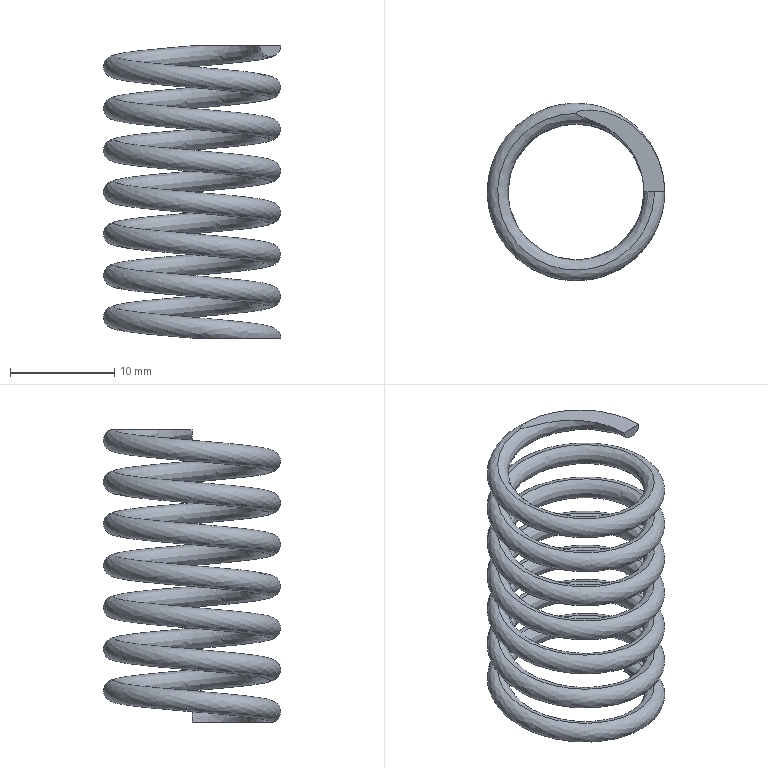Part | SolidWorks | features Split 2, Helix 1, Sweep 1 | 1 solid | 6 faces | box 17 x 17 x 28 mm | volume 1021 mm3 | plane 4 | spline 2